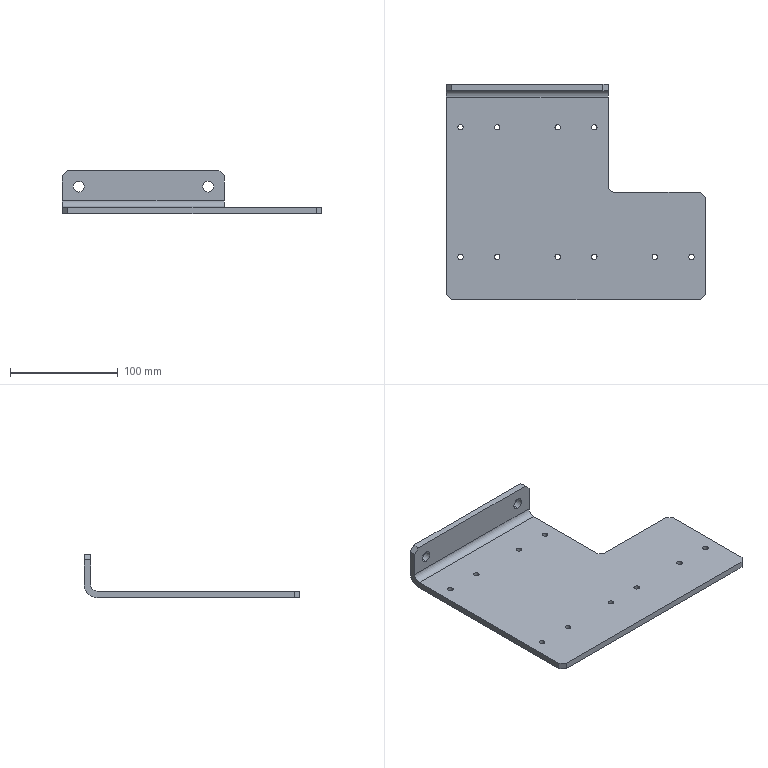Part | STEP file | [01]-7 | 1 solid | 42 faces | box 240 x 200 x 40 mm | volume 258660 mm3 | cylinder 27 | plane 15 | commonest cylinder face diameters 5 x20 10 x5 12 x1 24 x1